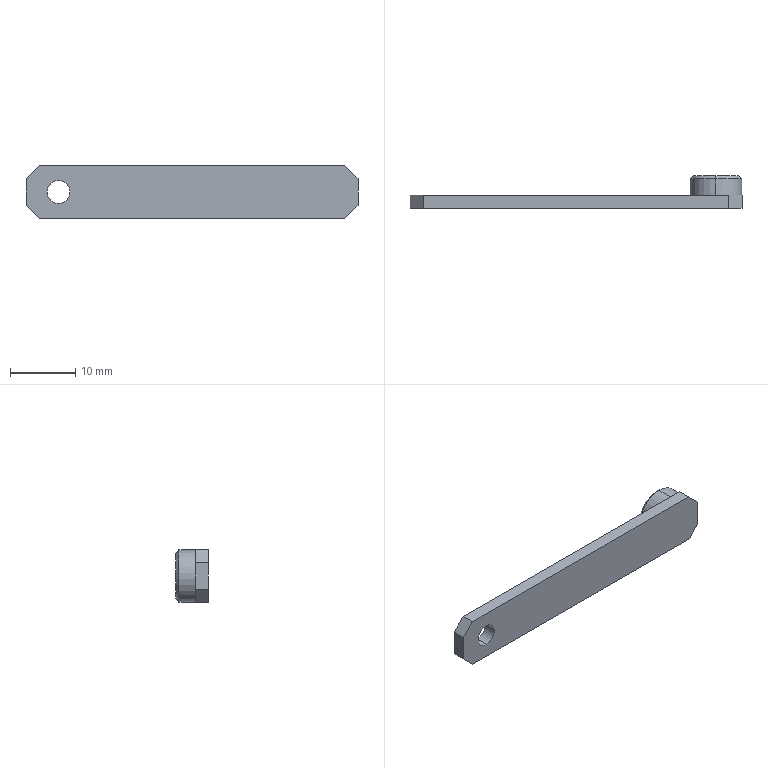Part | SolidWorks | features Chamfer 2, ICE 2, Extrusion 1 | 1 solid | 19 faces | box 51 x 5 x 8 mm | volume 928.543 mm3 | plane 13 | cylinder 4 | cone 2 | commonest cylinder face diameters 3.5 x2 8 x2
STEP:
#1=CARTESIAN_POINT('',(47.,5.,-0.5));
#2=VERTEX_POINT('',#1);
#3=CARTESIAN_POINT('',(47.,5.,-7.5));
#4=VERTEX_POINT('',#3);
#5=CARTESIAN_POINT('',(47.,5.,-4.));
#6=DIRECTION('',(0.,1.,0.));
#7=DIRECTION('',(0.,0.,1.));
#8=AXIS2_PLACEMENT_3D('',#5,#6,#7);
#9=CIRCLE('',#8,3.5);
#10=EDGE_CURVE('',#2,#4,#9,.T.);
#11=ORIENTED_EDGE('',*,*,#10,.F.);
#12=CARTESIAN_POINT('',(47.,4.5,0.));
#13=VERTEX_POINT('',#12);
#14=CARTESIAN_POINT('',(47.,5.,-0.5));
#15=DIRECTION('',(0.,-0.7071,0.7071));
#16=VECTOR('',#15,1000.);
#17=LINE('',#14,#16);
#18=EDGE_CURVE('',#2,#13,#17,.T.);
#19=ORIENTED_EDGE('',*,*,#18,.T.);
#20=CARTESIAN_POINT('',(47.,4.5,-8.));
#21=VERTEX_POINT('',#20);
#22=CARTESIAN_POINT('',(47.,4.5,-4.));
#23=DIRECTION('',(0.,-1.,0.));
#24=DIRECTION('',(0.,0.,1.));
#25=AXIS2_PLACEMENT_3D('',#22,#23,#24);
#26=CIRCLE('',#25,4.);
#27=EDGE_CURVE('',#21,#13,#26,.T.);
#28=ORIENTED_EDGE('',*,*,#27,.F.);
#29=CARTESIAN_POINT('',(47.,5.,-7.5));
#30=DIRECTION('',(0.,-0.7071,-0.7071));
#31=VECTOR('',#30,1000.);
#32=LINE('',#29,#31);
#33=EDGE_CURVE('',#4,#21,#32,.T.);
#34=ORIENTED_EDGE('',*,*,#33,.F.);
#35=EDGE_LOOP('',(#11,#19,#28,#34));
#36=FACE_OUTER_BOUND('',#35,.T.);
#37=CARTESIAN_POINT('',(47.,5.,-4.));
#38=DIRECTION('',(0.,-1.,0.));
#39=DIRECTION('',(0.,0.,-1.));
#40=AXIS2_PLACEMENT_3D('',#37,#38,#39);
#41=CONICAL_SURFACE('',#40,3.5,0.7854);
#42=ADVANCED_FACE('',(#36),#41,.T.);
#43=ORIENTED_EDGE('',*,*,#27,.T.);
#44=CARTESIAN_POINT('',(47.,2.,0.));
#45=VERTEX_POINT('',#44);
#46=CARTESIAN_POINT('',(47.,5.,0.));
#47=DIRECTION('',(0.,-1.,0.));
#48=VECTOR('',#47,1000.);
#49=LINE('',#46,#48);
#50=EDGE_CURVE('',#13,#45,#49,.T.);
#51=ORIENTED_EDGE('',*,*,#50,.T.);
#52=CARTESIAN_POINT('',(51.,2.,-4.));
#53=VERTEX_POINT('',#52);
#54=CARTESIAN_POINT('',(47.,2.,-4.));
#55=DIRECTION('',(0.,1.,0.));
#56=DIRECTION('',(0.,0.,1.));
#57=AXIS2_PLACEMENT_3D('',#54,#55,#56);
#58=CIRCLE('',#57,4.);
#59=EDGE_CURVE('',#45,#53,#58,.T.);
#60=ORIENTED_EDGE('',*,*,#59,.T.);
#61=CARTESIAN_POINT('',(47.,2.,-8.));
#62=VERTEX_POINT('',#61);
#63=CARTESIAN_POINT('',(47.,2.,-4.));
#64=DIRECTION('',(0.,1.,0.));
#65=DIRECTION('',(0.,0.,1.));
#66=AXIS2_PLACEMENT_3D('',#63,#64,#65);
#67=CIRCLE('',#66,4.);
#68=EDGE_CURVE('',#53,#62,#67,.T.);
#69=ORIENTED_EDGE('',*,*,#68,.T.);
#70=CARTESIAN_POINT('',(47.,5.,-8.));
#71=DIRECTION('',(0.,-1.,0.));
#72=VECTOR('',#71,1000.);
#73=LINE('',#70,#72);
#74=EDGE_CURVE('',#21,#62,#73,.T.);
#75=ORIENTED_EDGE('',*,*,#74,.F.);
#76=EDGE_LOOP('',(#43,#51,#60,#69,#75));
#77=FACE_OUTER_BOUND('',#76,.T.);
#78=CARTESIAN_POINT('',(47.,5.,-4.));
#79=DIRECTION('',(0.,-1.,0.));
#80=DIRECTION('',(0.,0.,-1.));
#81=AXIS2_PLACEMENT_3D('',#78,#79,#80);
#82=CYLINDRICAL_SURFACE('',#81,4.);
#83=ADVANCED_FACE('',(#77),#82,.T.);
#84=CARTESIAN_POINT('',(5.,0.,-5.75));
#85=VERTEX_POINT('',#84);
#86=CARTESIAN_POINT('',(5.,0.,-2.25));
#87=VERTEX_POINT('',#86);
#88=CARTESIAN_POINT('',(5.,0.,-4.));
#89=DIRECTION('',(0.,1.,0.));
#90=DIRECTION('',(0.,0.,1.));
#91=AXIS2_PLACEMENT_3D('',#88,#89,#90);
#92=CIRCLE('',#91,1.75);
#93=EDGE_CURVE('',#85,#87,#92,.T.);
#94=ORIENTED_EDGE('',*,*,#93,.F.);
#95=CARTESIAN_POINT('',(5.,2.,-5.75));
#96=VERTEX_POINT('',#95);
#97=CARTESIAN_POINT('',(5.,0.,-5.75));
#98=DIRECTION('',(0.,1.,0.));
#99=VECTOR('',#98,1000.);
#100=LINE('',#97,#99);
#101=EDGE_CURVE('',#85,#96,#100,.T.);
#102=ORIENTED_EDGE('',*,*,#101,.T.);
#103=CARTESIAN_POINT('',(5.,2.,-2.25));
#104=VERTEX_POINT('',#103);
#105=CARTESIAN_POINT('',(5.,2.,-4.));
#106=DIRECTION('',(0.,1.,0.));
#107=DIRECTION('',(0.,0.,1.));
#108=AXIS2_PLACEMENT_3D('',#105,#106,#107);
#109=CIRCLE('',#108,1.75);
#110=EDGE_CURVE('',#96,#104,#109,.T.);
#111=ORIENTED_EDGE('',*,*,#110,.T.);
#112=CARTESIAN_POINT('',(5.,0.,-2.25));
#113=DIRECTION('',(0.,1.,0.));
#114=VECTOR('',#113,1000.);
#115=LINE('',#112,#114);
#116=EDGE_CURVE('',#87,#104,#115,.T.);
#117=ORIENTED_EDGE('',*,*,#116,.F.);
#118=EDGE_LOOP('',(#94,#102,#111,#117));
#119=FACE_OUTER_BOUND('',#118,.T.);
#120=CARTESIAN_POINT('',(5.,0.,-4.));
#121=DIRECTION('',(0.,1.,0.));
#122=DIRECTION('',(0.,0.,1.));
#123=AXIS2_PLACEMENT_3D('',#120,#121,#122);
#124=CYLINDRICAL_SURFACE('',#123,1.75);
#125=ADVANCED_FACE('',(#119),#124,.F.);
#126=CARTESIAN_POINT('',(49.,2.,0.));
#127=VERTEX_POINT('',#126);
#128=CARTESIAN_POINT('',(0.,2.,0.));
#129=DIRECTION('',(1.,0.,0.));
#130=VECTOR('',#129,1000.);
#131=LINE('',#128,#130);
#132=EDGE_CURVE('',#45,#127,#131,.T.);
#133=ORIENTED_EDGE('',*,*,#132,.T.);
#134=CARTESIAN_POINT('',(51.,2.,-2.));
#135=VERTEX_POINT('',#134);
#136=CARTESIAN_POINT('',(24.5,2.,24.5));
#137=DIRECTION('',(0.7071,0.,-0.7071));
#138=VECTOR('',#137,1000.);
#139=LINE('',#136,#138);
#140=EDGE_CURVE('',#127,#135,#139,.T.);
#141=ORIENTED_EDGE('',*,*,#140,.T.);
#142=CARTESIAN_POINT('',(51.,2.,-8.));
#143=DIRECTION('',(0.,0.,-1.));
#144=VECTOR('',#143,1000.);
#145=LINE('',#142,#144);
#146=EDGE_CURVE('',#135,#53,#145,.T.);
#147=ORIENTED_EDGE('',*,*,#146,.T.);
#148=ORIENTED_EDGE('',*,*,#59,.F.);
#149=EDGE_LOOP('',(#133,#141,#147,#148));
#150=FACE_OUTER_BOUND('',#149,.T.);
#151=CARTESIAN_POINT('',(0.,2.,0.));
#152=DIRECTION('',(0.,1.,0.));
#153=DIRECTION('',(0.,0.,1.));
#154=AXIS2_PLACEMENT_3D('',#151,#152,#153);
#155=PLANE('',#154);
#156=ADVANCED_FACE('',(#150),#155,.T.);
#157=CARTESIAN_POINT('',(51.,2.,-6.));
#158=VERTEX_POINT('',#157);
#159=CARTESIAN_POINT('',(51.,2.,-8.));
#160=DIRECTION('',(0.,0.,-1.));
#161=VECTOR('',#160,1000.);
#162=LINE('',#159,#161);
#163=EDGE_CURVE('',#53,#158,#162,.T.);
#164=ORIENTED_EDGE('',*,*,#163,.T.);
#165=CARTESIAN_POINT('',(49.,2.,-8.));
#166=VERTEX_POINT('',#165);
#167=CARTESIAN_POINT('',(28.5,2.,-28.5));
#168=DIRECTION('',(-0.7071,0.,-0.7071));
#169=VECTOR('',#168,1000.);
#170=LINE('',#167,#169);
#171=EDGE_CURVE('',#158,#166,#170,.T.);
#172=ORIENTED_EDGE('',*,*,#171,.T.);
#173=CARTESIAN_POINT('',(0.,2.,-8.));
#174=DIRECTION('',(-1.,0.,0.));
#175=VECTOR('',#174,1000.);
#176=LINE('',#173,#175);
#177=EDGE_CURVE('',#166,#62,#176,.T.);
#178=ORIENTED_EDGE('',*,*,#177,.T.);
#179=ORIENTED_EDGE('',*,*,#68,.F.);
#180=EDGE_LOOP('',(#164,#172,#178,#179));
#181=FACE_OUTER_BOUND('',#180,.T.);
#182=CARTESIAN_POINT('',(0.,2.,0.));
#183=DIRECTION('',(0.,1.,0.));
#184=DIRECTION('',(0.,0.,1.));
#185=AXIS2_PLACEMENT_3D('',#182,#183,#184);
#186=PLANE('',#185);
#187=ADVANCED_FACE('',(#181),#186,.T.);
#188=CARTESIAN_POINT('',(0.,2.,-6.));
#189=VERTEX_POINT('',#188);
#190=CARTESIAN_POINT('',(0.,2.,-2.));
#191=VERTEX_POINT('',#190);
#192=CARTESIAN_POINT('',(0.,2.,-8.));
#193=DIRECTION('',(0.,0.,1.));
#194=VECTOR('',#193,1000.);
#195=LINE('',#192,#194);
#196=EDGE_CURVE('',#189,#191,#195,.T.);
#197=ORIENTED_EDGE('',*,*,#196,.F.);
#198=CARTESIAN_POINT('',(0.,0.,-6.));
#199=VERTEX_POINT('',#198);
#200=CARTESIAN_POINT('',(0.,2.,-6.));
#201=DIRECTION('',(0.,-1.,0.));
#202=VECTOR('',#201,1000.);
#203=LINE('',#200,#202);
#204=EDGE_CURVE('',#189,#199,#203,.T.);
#205=ORIENTED_EDGE('',*,*,#204,.T.);
#206=CARTESIAN_POINT('',(0.,0.,-2.));
#207=VERTEX_POINT('',#206);
#208=CARTESIAN_POINT('',(0.,0.,-8.));
#209=DIRECTION('',(0.,0.,1.));
#210=VECTOR('',#209,1000.);
#211=LINE('',#208,#210);
#212=EDGE_CURVE('',#199,#207,#211,.T.);
#213=ORIENTED_EDGE('',*,*,#212,.T.);
#214=CARTESIAN_POINT('',(0.,2.,-2.));
#215=DIRECTION('',(0.,1.,0.));
#216=VECTOR('',#215,1000.);
#217=LINE('',#214,#216);
#218=EDGE_CURVE('',#207,#191,#217,.T.);
#219=ORIENTED_EDGE('',*,*,#218,.T.);
#220=EDGE_LOOP('',(#197,#205,#213,#219));
#221=FACE_OUTER_BOUND('',#220,.T.);
#222=CARTESIAN_POINT('',(0.,2.,-8.));
#223=DIRECTION('',(1.,0.,0.));
#224=DIRECTION('',(0.,0.,-1.));
#225=AXIS2_PLACEMENT_3D('',#222,#223,#224);
#226=PLANE('',#225);
#227=ADVANCED_FACE('',(#221),#226,.F.);
#228=CARTESIAN_POINT('',(2.,0.,0.));
#229=VERTEX_POINT('',#228);
#230=CARTESIAN_POINT('',(49.,0.,0.));
#231=VERTEX_POINT('',#230);
#232=CARTESIAN_POINT('',(0.,0.,0.));
#233=DIRECTION('',(1.,0.,0.));
#234=VECTOR('',#233,1000.);
#235=LINE('',#232,#234);
#236=EDGE_CURVE('',#229,#231,#235,.T.);
#237=ORIENTED_EDGE('',*,*,#236,.T.);
#238=CARTESIAN_POINT('',(49.,2.,0.));
#239=DIRECTION('',(0.,1.,0.));
#240=VECTOR('',#239,1000.);
#241=LINE('',#238,#240);
#242=EDGE_CURVE('',#231,#127,#241,.T.);
#243=ORIENTED_EDGE('',*,*,#242,.T.);
#244=ORIENTED_EDGE('',*,*,#132,.F.);
#245=CARTESIAN_POINT('',(2.,2.,0.));
#246=VERTEX_POINT('',#245);
#247=CARTESIAN_POINT('',(0.,2.,0.));
#248=DIRECTION('',(1.,0.,0.));
#249=VECTOR('',#248,1000.);
#250=LINE('',#247,#249);
#251=EDGE_CURVE('',#246,#45,#250,.T.);
#252=ORIENTED_EDGE('',*,*,#251,.F.);
#253=CARTESIAN_POINT('',(2.,2.,0.));
#254=DIRECTION('',(0.,-1.,0.));
#255=VECTOR('',#254,1000.);
#256=LINE('',#253,#255);
#257=EDGE_CURVE('',#246,#229,#256,.T.);
#258=ORIENTED_EDGE('',*,*,#257,.T.);
#259=EDGE_LOOP('',(#237,#243,#244,#252,#258));
#260=FACE_OUTER_BOUND('',#259,.T.);
#261=CARTESIAN_POINT('',(0.,2.,0.));
#262=DIRECTION('',(0.,0.,-1.));
#263=DIRECTION('',(-1.,0.,0.));
#264=AXIS2_PLACEMENT_3D('',#261,#262,#263);
#265=PLANE('',#264);
#266=ADVANCED_FACE('',(#260),#265,.F.);
#267=CARTESIAN_POINT('',(51.,0.,-2.));
#268=VERTEX_POINT('',#267);
#269=CARTESIAN_POINT('',(51.,0.,-6.));
#270=VERTEX_POINT('',#269);
#271=CARTESIAN_POINT('',(51.,0.,-8.));
#272=DIRECTION('',(0.,0.,-1.));
#273=VECTOR('',#272,1000.);
#274=LINE('',#271,#273);
#275=EDGE_CURVE('',#268,#270,#274,.T.);
#276=ORIENTED_EDGE('',*,*,#275,.T.);
#277=CARTESIAN_POINT('',(51.,2.,-6.));
#278=DIRECTION('',(0.,1.,0.));
#279=VECTOR('',#278,1000.);
#280=LINE('',#277,#279);
#281=EDGE_CURVE('',#270,#158,#280,.T.);
#282=ORIENTED_EDGE('',*,*,#281,.T.);
#283=ORIENTED_EDGE('',*,*,#163,.F.);
#284=ORIENTED_EDGE('',*,*,#146,.F.);
#285=CARTESIAN_POINT('',(51.,2.,-2.));
#286=DIRECTION('',(0.,-1.,0.));
#287=VECTOR('',#286,1000.);
#288=LINE('',#285,#287);
#289=EDGE_CURVE('',#135,#268,#288,.T.);
#290=ORIENTED_EDGE('',*,*,#289,.T.);
#291=EDGE_LOOP('',(#276,#282,#283,#284,#290));
#292=FACE_OUTER_BOUND('',#291,.T.);
#293=CARTESIAN_POINT('',(51.,2.,-8.));
#294=DIRECTION('',(-1.,0.,0.));
#295=DIRECTION('',(0.,0.,1.));
#296=AXIS2_PLACEMENT_3D('',#293,#294,#295);
#297=PLANE('',#296);
#298=ADVANCED_FACE('',(#292),#297,.F.);
#299=ORIENTED_EDGE('',*,*,#177,.F.);
#300=CARTESIAN_POINT('',(49.,0.,-8.));
#301=VERTEX_POINT('',#300);
#302=CARTESIAN_POINT('',(49.,2.,-8.));
#303=DIRECTION('',(0.,-1.,0.));
#304=VECTOR('',#303,1000.);
#305=LINE('',#302,#304);
#306=EDGE_CURVE('',#166,#301,#305,.T.);
#307=ORIENTED_EDGE('',*,*,#306,.T.);
#308=CARTESIAN_POINT('',(2.,0.,-8.));
#309=VERTEX_POINT('',#308);
#310=CARTESIAN_POINT('',(0.,0.,-8.));
#311=DIRECTION('',(-1.,0.,0.));
#312=VECTOR('',#311,1000.);
#313=LINE('',#310,#312);
#314=EDGE_CURVE('',#301,#309,#313,.T.);
#315=ORIENTED_EDGE('',*,*,#314,.T.);
#316=CARTESIAN_POINT('',(2.,2.,-8.));
#317=VERTEX_POINT('',#316);
#318=CARTESIAN_POINT('',(2.,2.,-8.));
#319=DIRECTION('',(0.,1.,0.));
#320=VECTOR('',#319,1000.);
#321=LINE('',#318,#320);
#322=EDGE_CURVE('',#309,#317,#321,.T.);
#323=ORIENTED_EDGE('',*,*,#322,.T.);
#324=CARTESIAN_POINT('',(0.,2.,-8.));
#325=DIRECTION('',(-1.,0.,0.));
#326=VECTOR('',#325,1000.);
#327=LINE('',#324,#326);
#328=EDGE_CURVE('',#62,#317,#327,.T.);
#329=ORIENTED_EDGE('',*,*,#328,.F.);
#330=EDGE_LOOP('',(#299,#307,#315,#323,#329));
#331=FACE_OUTER_BOUND('',#330,.T.);
#332=CARTESIAN_POINT('',(0.,2.,-8.));
#333=DIRECTION('',(0.,0.,1.));
#334=DIRECTION('',(1.,0.,0.));
#335=AXIS2_PLACEMENT_3D('',#332,#333,#334);
#336=PLANE('',#335);
#337=ADVANCED_FACE('',(#331),#336,.F.);
#338=ORIENTED_EDGE('',*,*,#328,.T.);
#339=CARTESIAN_POINT('',(-3.,2.,-3.));
#340=DIRECTION('',(-0.7071,0.,0.7071));
#341=VECTOR('',#340,1000.);
#342=LINE('',#339,#341);
#343=EDGE_CURVE('',#317,#189,#342,.T.);
#344=ORIENTED_EDGE('',*,*,#343,.T.);
#345=ORIENTED_EDGE('',*,*,#196,.T.);
#346=CARTESIAN_POINT('',(1.,2.,-1.));
#347=DIRECTION('',(0.7071,0.,0.7071));
#348=VECTOR('',#347,1000.);
#349=LINE('',#346,#348);
#350=EDGE_CURVE('',#191,#246,#349,.T.);
#351=ORIENTED_EDGE('',*,*,#350,.T.);
#352=ORIENTED_EDGE('',*,*,#251,.T.);
#353=CARTESIAN_POINT('',(47.,2.,-4.));
#354=DIRECTION('',(0.,1.,0.));
#355=DIRECTION('',(0.,0.,1.));
#356=AXIS2_PLACEMENT_3D('',#353,#354,#355);
#357=CIRCLE('',#356,4.);
#358=EDGE_CURVE('',#62,#45,#357,.T.);
#359=ORIENTED_EDGE('',*,*,#358,.F.);
#360=EDGE_LOOP('',(#338,#344,#345,#351,#352,#359));
#361=FACE_OUTER_BOUND('',#360,.T.);
#362=CARTESIAN_POINT('',(5.,2.,-4.));
#363=DIRECTION('',(0.,1.,0.));
#364=DIRECTION('',(0.,0.,1.));
#365=AXIS2_PLACEMENT_3D('',#362,#363,#364);
#366=CIRCLE('',#365,1.75);
#367=EDGE_CURVE('',#104,#96,#366,.T.);
#368=ORIENTED_EDGE('',*,*,#367,.F.);
#369=ORIENTED_EDGE('',*,*,#110,.F.);
#370=EDGE_LOOP('',(#368,#369));
#371=FACE_BOUND('',#370,.T.);
#372=CARTESIAN_POINT('',(0.,2.,0.));
#373=DIRECTION('',(0.,1.,0.));
#374=DIRECTION('',(0.,0.,1.));
#375=AXIS2_PLACEMENT_3D('',#372,#373,#374);
#376=PLANE('',#375);
#377=ADVANCED_FACE('',(#361,#371),#376,.T.);
#378=CARTESIAN_POINT('',(5.,0.,-4.));
#379=DIRECTION('',(0.,1.,0.));
#380=DIRECTION('',(0.,0.,1.));
#381=AXIS2_PLACEMENT_3D('',#378,#379,#380);
#382=CIRCLE('',#381,1.75);
#383=EDGE_CURVE('',#87,#85,#382,.T.);
#384=ORIENTED_EDGE('',*,*,#383,.T.);
#385=ORIENTED_EDGE('',*,*,#93,.T.);
#386=EDGE_LOOP('',(#384,#385));
#387=FACE_BOUND('',#386,.T.);
#388=ORIENTED_EDGE('',*,*,#314,.F.);
#389=CARTESIAN_POINT('',(49.,0.,-8.));
#390=DIRECTION('',(0.7071,0.,0.7071));
#391=VECTOR('',#390,1000.);
#392=LINE('',#389,#391);
#393=EDGE_CURVE('',#301,#270,#392,.T.);
#394=ORIENTED_EDGE('',*,*,#393,.T.);
#395=ORIENTED_EDGE('',*,*,#275,.F.);
#396=CARTESIAN_POINT('',(51.,0.,-2.));
#397=DIRECTION('',(-0.7071,0.,0.7071));
#398=VECTOR('',#397,1000.);
#399=LINE('',#396,#398);
#400=EDGE_CURVE('',#268,#231,#399,.T.);
#401=ORIENTED_EDGE('',*,*,#400,.T.);
#402=ORIENTED_EDGE('',*,*,#236,.F.);
#403=CARTESIAN_POINT('',(2.,0.,0.));
#404=DIRECTION('',(-0.7071,0.,-0.7071));
#405=VECTOR('',#404,1000.);
#406=LINE('',#403,#405);
#407=EDGE_CURVE('',#229,#207,#406,.T.);
#408=ORIENTED_EDGE('',*,*,#407,.T.);
#409=ORIENTED_EDGE('',*,*,#212,.F.);
#410=CARTESIAN_POINT('',(0.,0.,-6.));
#411=DIRECTION('',(0.7071,0.,-0.7071));
#412=VECTOR('',#411,1000.);
#413=LINE('',#410,#412);
#414=EDGE_CURVE('',#199,#309,#413,.T.);
#415=ORIENTED_EDGE('',*,*,#414,.T.);
#416=EDGE_LOOP('',(#388,#394,#395,#401,#402,#408,#409,#415));
#417=FACE_OUTER_BOUND('',#416,.T.);
#418=CARTESIAN_POINT('',(0.,0.,0.));
#419=DIRECTION('',(0.,1.,0.));
#420=DIRECTION('',(0.,0.,1.));
#421=AXIS2_PLACEMENT_3D('',#418,#419,#420);
#422=PLANE('',#421);
#423=ADVANCED_FACE('',(#387,#417),#422,.F.);
#424=ORIENTED_EDGE('',*,*,#101,.F.);
#425=ORIENTED_EDGE('',*,*,#383,.F.);
#426=ORIENTED_EDGE('',*,*,#116,.T.);
#427=ORIENTED_EDGE('',*,*,#367,.T.);
#428=EDGE_LOOP('',(#424,#425,#426,#427));
#429=FACE_OUTER_BOUND('',#428,.T.);
#430=CARTESIAN_POINT('',(5.,0.,-4.));
#431=DIRECTION('',(0.,1.,0.));
#432=DIRECTION('',(0.,0.,1.));
#433=AXIS2_PLACEMENT_3D('',#430,#431,#432);
#434=CYLINDRICAL_SURFACE('',#433,1.75);
#435=ADVANCED_FACE('',(#429),#434,.F.);
#436=ORIENTED_EDGE('',*,*,#50,.F.);
#437=CARTESIAN_POINT('',(47.,4.5,-4.));
#438=DIRECTION('',(0.,-1.,0.));
#439=DIRECTION('',(0.,0.,1.));
#440=AXIS2_PLACEMENT_3D('',#437,#438,#439);
#441=CIRCLE('',#440,4.);
#442=EDGE_CURVE('',#13,#21,#441,.T.);
#443=ORIENTED_EDGE('',*,*,#442,.T.);
#444=ORIENTED_EDGE('',*,*,#74,.T.);
#445=ORIENTED_EDGE('',*,*,#358,.T.);
#446=EDGE_LOOP('',(#436,#443,#444,#445));
#447=FACE_OUTER_BOUND('',#446,.T.);
#448=CARTESIAN_POINT('',(47.,5.,-4.));
#449=DIRECTION('',(0.,-1.,0.));
#450=DIRECTION('',(0.,0.,-1.));
#451=AXIS2_PLACEMENT_3D('',#448,#449,#450);
#452=CYLINDRICAL_SURFACE('',#451,4.);
#453=ADVANCED_FACE('',(#447),#452,.T.);
#454=CARTESIAN_POINT('',(47.,5.,-4.));
#455=DIRECTION('',(0.,1.,0.));
#456=DIRECTION('',(0.,0.,1.));
#457=AXIS2_PLACEMENT_3D('',#454,#455,#456);
#458=CIRCLE('',#457,3.5);
#459=EDGE_CURVE('',#4,#2,#458,.T.);
#460=ORIENTED_EDGE('',*,*,#459,.T.);
#461=ORIENTED_EDGE('',*,*,#10,.T.);
#462=EDGE_LOOP('',(#460,#461));
#463=FACE_OUTER_BOUND('',#462,.T.);
#464=CARTESIAN_POINT('',(47.,5.,-4.));
#465=DIRECTION('',(0.,1.,0.));
#466=DIRECTION('',(0.,0.,1.));
#467=AXIS2_PLACEMENT_3D('',#464,#465,#466);
#468=PLANE('',#467);
#469=ADVANCED_FACE('',(#463),#468,.T.);
#470=ORIENTED_EDGE('',*,*,#18,.F.);
#471=ORIENTED_EDGE('',*,*,#459,.F.);
#472=ORIENTED_EDGE('',*,*,#33,.T.);
#473=ORIENTED_EDGE('',*,*,#442,.F.);
#474=EDGE_LOOP('',(#470,#471,#472,#473));
#475=FACE_OUTER_BOUND('',#474,.T.);
#476=CARTESIAN_POINT('',(47.,5.,-4.));
#477=DIRECTION('',(0.,-1.,0.));
#478=DIRECTION('',(0.,0.,-1.));
#479=AXIS2_PLACEMENT_3D('',#476,#477,#478);
#480=CONICAL_SURFACE('',#479,3.5,0.7854);
#481=ADVANCED_FACE('',(#475),#480,.T.);
#482=ORIENTED_EDGE('',*,*,#171,.F.);
#483=ORIENTED_EDGE('',*,*,#281,.F.);
#484=ORIENTED_EDGE('',*,*,#393,.F.);
#485=ORIENTED_EDGE('',*,*,#306,.F.);
#486=EDGE_LOOP('',(#482,#483,#484,#485));
#487=FACE_OUTER_BOUND('',#486,.T.);
#488=CARTESIAN_POINT('',(49.,2.,-8.));
#489=DIRECTION('',(-0.7071,0.,0.7071));
#490=DIRECTION('',(0.,-1.,0.));
#491=AXIS2_PLACEMENT_3D('',#488,#489,#490);
#492=PLANE('',#491);
#493=ADVANCED_FACE('',(#487),#492,.F.);
#494=ORIENTED_EDGE('',*,*,#140,.F.);
#495=ORIENTED_EDGE('',*,*,#242,.F.);
#496=ORIENTED_EDGE('',*,*,#400,.F.);
#497=ORIENTED_EDGE('',*,*,#289,.F.);
#498=EDGE_LOOP('',(#494,#495,#496,#497));
#499=FACE_OUTER_BOUND('',#498,.T.);
#500=CARTESIAN_POINT('',(51.,2.,-2.));
#501=DIRECTION('',(-0.7071,0.,-0.7071));
#502=DIRECTION('',(0.,-1.,0.));
#503=AXIS2_PLACEMENT_3D('',#500,#501,#502);
#504=PLANE('',#503);
#505=ADVANCED_FACE('',(#499),#504,.F.);
#506=ORIENTED_EDGE('',*,*,#343,.F.);
#507=ORIENTED_EDGE('',*,*,#322,.F.);
#508=ORIENTED_EDGE('',*,*,#414,.F.);
#509=ORIENTED_EDGE('',*,*,#204,.F.);
#510=EDGE_LOOP('',(#506,#507,#508,#509));
#511=FACE_OUTER_BOUND('',#510,.T.);
#512=CARTESIAN_POINT('',(0.,2.,-6.));
#513=DIRECTION('',(0.7071,0.,0.7071));
#514=DIRECTION('',(0.,-1.,0.));
#515=AXIS2_PLACEMENT_3D('',#512,#513,#514);
#516=PLANE('',#515);
#517=ADVANCED_FACE('',(#511),#516,.F.);
#518=ORIENTED_EDGE('',*,*,#350,.F.);
#519=ORIENTED_EDGE('',*,*,#218,.F.);
#520=ORIENTED_EDGE('',*,*,#407,.F.);
#521=ORIENTED_EDGE('',*,*,#257,.F.);
#522=EDGE_LOOP('',(#518,#519,#520,#521));
#523=FACE_OUTER_BOUND('',#522,.T.);
#524=CARTESIAN_POINT('',(2.,2.,0.));
#525=DIRECTION('',(0.7071,0.,-0.7071));
#526=DIRECTION('',(0.,-1.,0.));
#527=AXIS2_PLACEMENT_3D('',#524,#525,#526);
#528=PLANE('',#527);
#529=ADVANCED_FACE('',(#523),#528,.F.);
#530=CLOSED_SHELL('',(#42,#83,#125,#156,#187,#227,#266,#298,#337,#377,#423,#435,#453,#469,#481,#493,#505,#517,#529));
#531=MANIFOLD_SOLID_BREP('',#530);
#532=CARTESIAN_POINT('',(0.,0.,0.));
#533=DIRECTION('',(0.,0.,1.));
#534=DIRECTION('',(1.,0.,0.));
#535=AXIS2_PLACEMENT_3D('',#532,#533,#534);
#536=(LENGTH_UNIT()NAMED_UNIT(*)SI_UNIT(.MILLI.,.METRE.));
#537=UNCERTAINTY_MEASURE_WITH_UNIT(LENGTH_MEASURE(0.00001),#536,'','');
#538=(NAMED_UNIT(*)PLANE_ANGLE_UNIT()SI_UNIT($,.RADIAN.));
#539=(NAMED_UNIT(*)SI_UNIT($,.STERADIAN.)SOLID_ANGLE_UNIT());
#540=(GEOMETRIC_REPRESENTATION_CONTEXT(3)GLOBAL_UNCERTAINTY_ASSIGNED_CONTEXT((#537))GLOBAL_UNIT_ASSIGNED_CONTEXT((#536,#538,#539))REPRESENTATION_CONTEXT('',''));
#541=ADVANCED_BREP_SHAPE_REPRESENTATION('',(#531,#535),#540);